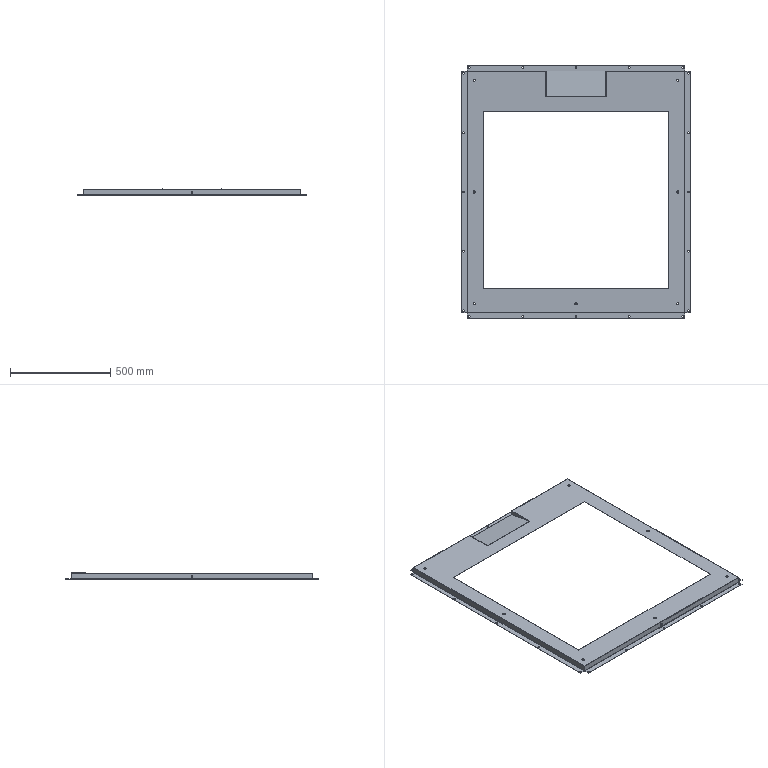Part | SolidWorks | 2 solids | 214 faces | box 1139 x 1259 x 30.281 mm | volume 733332 mm3 | plane 110 | cylinder 92 | spline 12 | commonest cylinder face diameters 7 x50 11 x14 0.4 x11 2.4 x11 10 x6